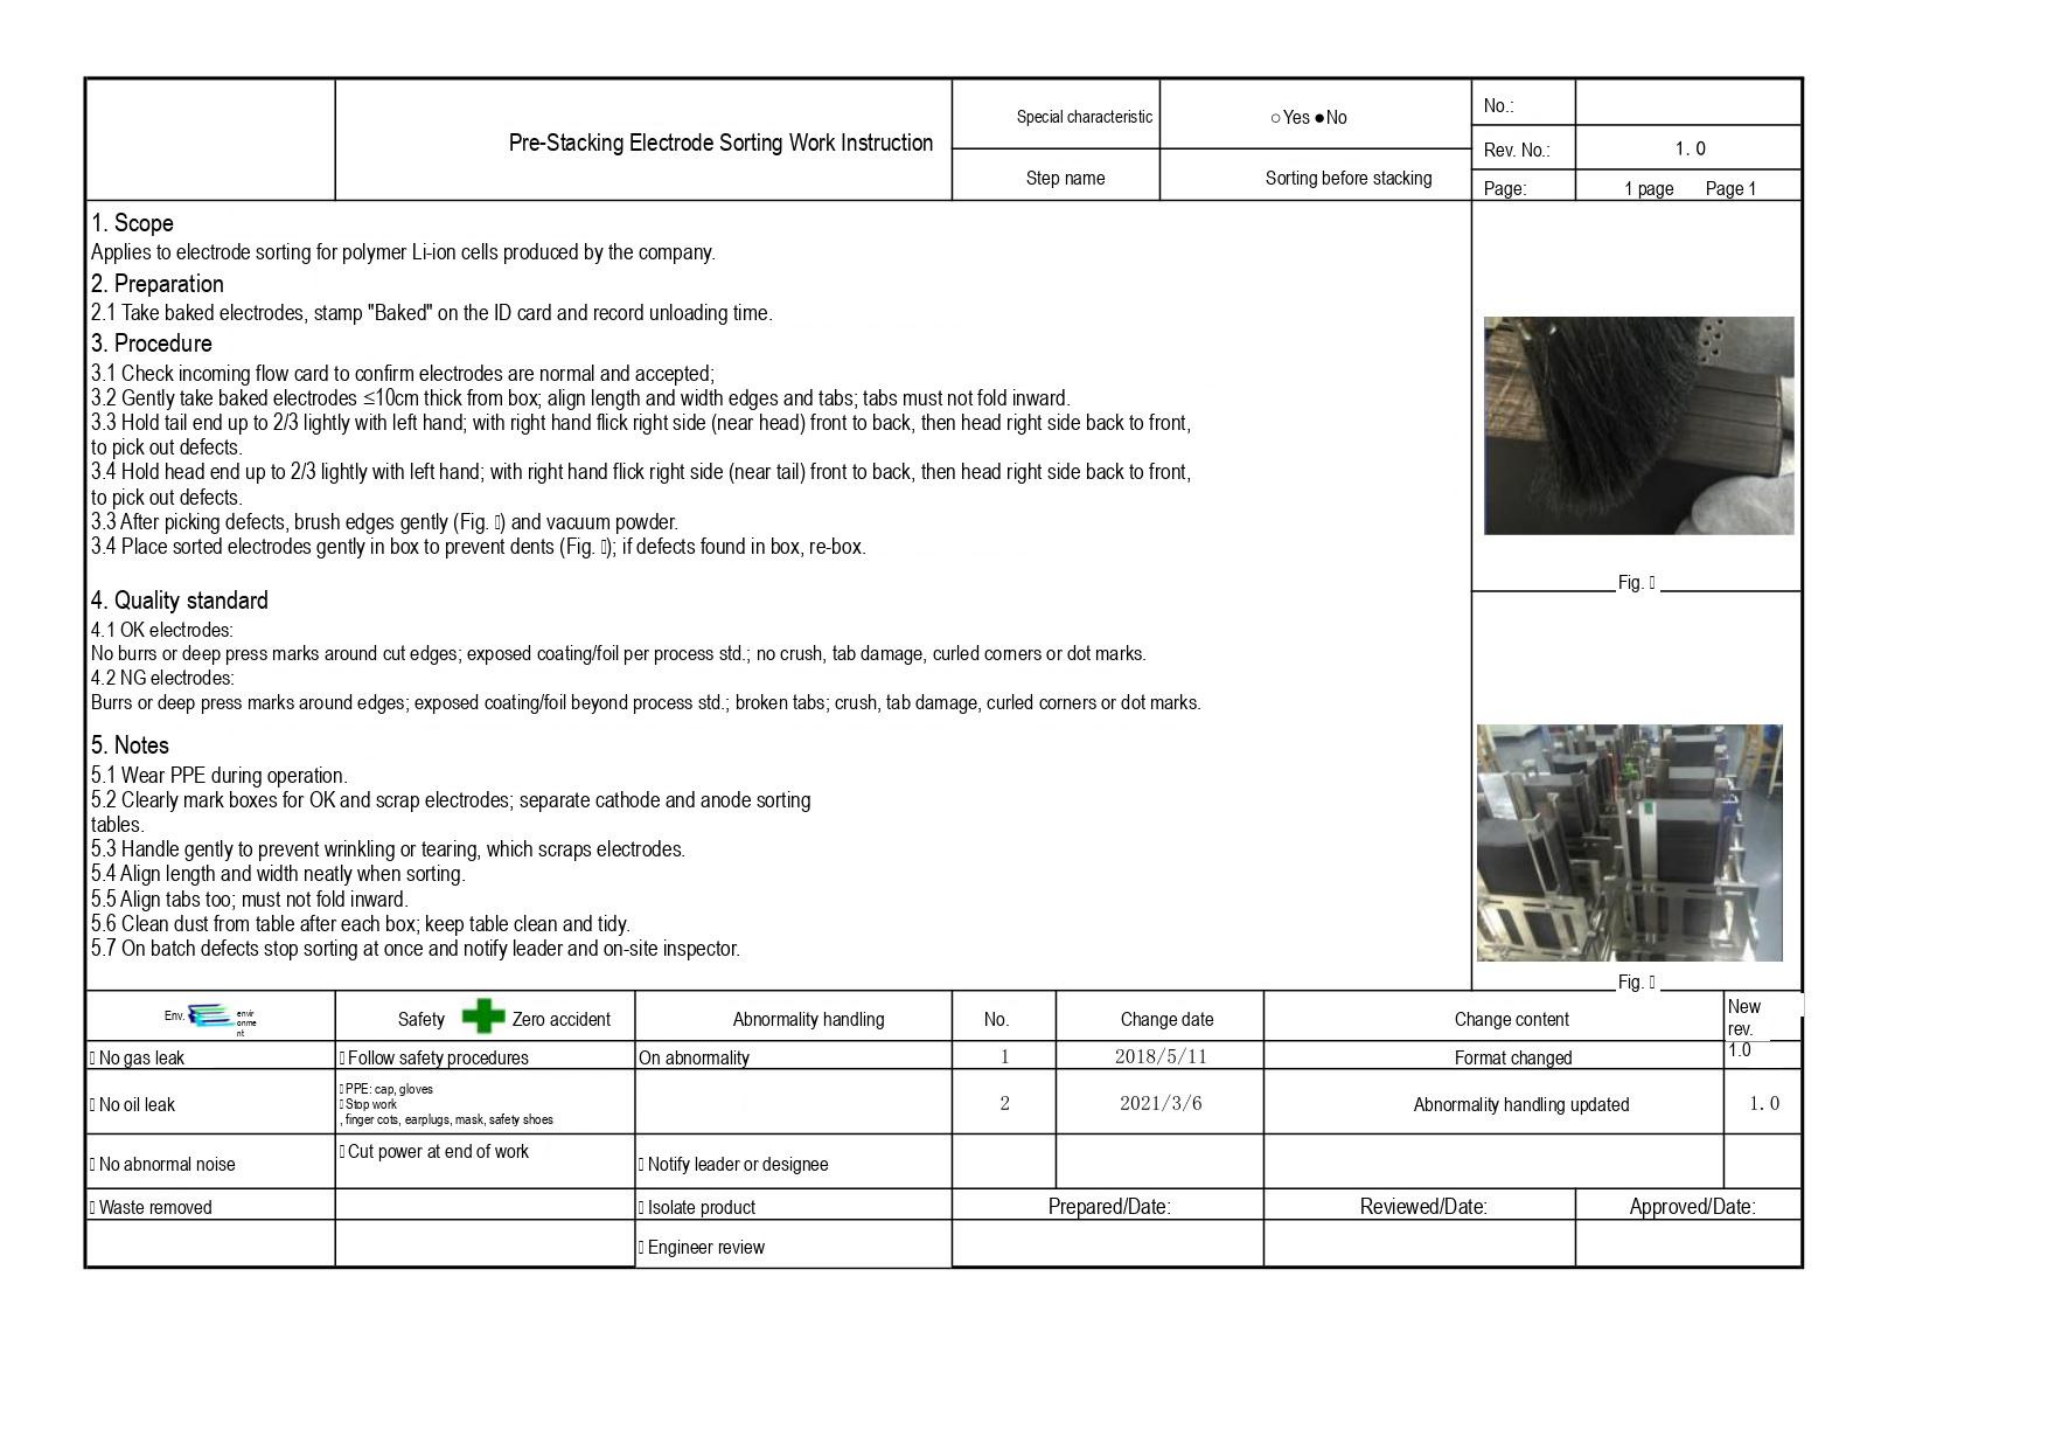| | Pre-Stacking Electrode Sorting Work Instruction | Special characteristic | ○Yes ●No | No.: | |
|---|---|---|---|---|---|
| | | Step name | Sorting before stacking | Rev. No.: | 1. 0 |
| | | | | Page: | 1 page Page 1 |

1. Scope
Applies to electrode sorting for polymer Li-ion cells produced by the company.
2. Preparation
2.1 Take baked electrodes, stamp "Baked" on the ID card and record unloading time.
3. Procedure
3.1 Check incoming flow card to confirm electrodes are normal and accepted;
3.2 Gently take baked electrodes ≤10cm thick from box; align length and width edges and tabs; tabs must not fold inward.
3.3 Hold tail end up to 2/3 lightly with left hand; with right hand flick right side (near head) front to back, then head right side back to front, to pick out defects.
3.4 Hold head end up to 2/3 lightly with left hand; with right hand flick right side (near tail) front to back, then head right side back to front, to pick out defects.
3.3 After picking defects, brush edges gently (Fig. ) and vacuum powder.
3.4 Place sorted electrodes gently in box to prevent dents (Fig. ); if defects found in box, re-box.

4. Quality standard
4.1 OK electrodes:
No burrs or deep press marks around cut edges; exposed coating/foil per process std.; no crush, tab damage, curled corners or dot marks.
4.2 NG electrodes:
Burrs or deep press marks around edges; exposed coating/foil beyond process std.; broken tabs; crush, tab damage, curled corners or dot marks.

5. Notes
5.1 Wear PPE during operation.
5.2 Clearly mark boxes for OK and scrap electrodes; separate cathode and anode sorting tables.
5.3 Handle gently to prevent wrinkling or tearing, which scraps electrodes.
5.4 Align length and width neatly when sorting.
5.5 Align tabs too; must not fold inward.
5.6 Clean dust from table after each box; keep table clean and tidy.
5.7 On batch defects stop sorting at once and notify leader and on-site inspector.

Fig.

Fig.

| Env. environment | Safety Zero accident | Abnormality handling | No. | Change date | Change content | New rev. |
|---|---|---|---|---|---|---|
| No gas leak | Follow safety procedures | On abnormality | 1 | 2018/5/11 | Format changed | 1.0 |
| No oil leak | PPE: cap, gloves<br>Stop work<br>, finger cots, earplugs, mask, safety shoes | | 2 | 2021/3/6 | Abnormality handling updated | 1. 0 |
| No abnormal noise | Cut power at end of work | Notify leader or designee | | | | |
| Waste removed | | Isolate product | Prepared/Date: | | Reviewed/Date: | Approved/Date: |
| | | Engineer review | | | | |